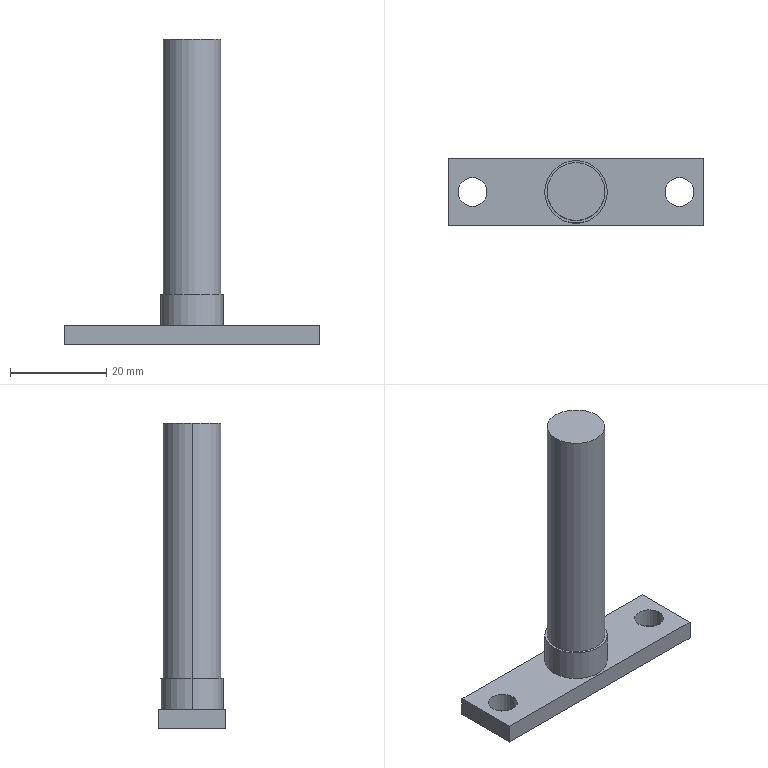Part | SolidWorks | features ICE 2, Extrusion 1 | 1 solid | 16 faces | box 53 x 14 x 63.5 mm | volume 9599 mm3 | cylinder 8 | plane 8 | commonest cylinder face diameters 6 x4 12 x2 13 x2
STEP:
#1=CARTESIAN_POINT('',(6.,0.,59.5));
#2=VERTEX_POINT('',#1);
#3=CARTESIAN_POINT('',(-6.,0.,59.5));
#4=VERTEX_POINT('',#3);
#5=CARTESIAN_POINT('',(0.,0.,59.5));
#6=DIRECTION('',(0.,0.,1.));
#7=DIRECTION('',(1.,0.,0.));
#8=AXIS2_PLACEMENT_3D('',#5,#6,#7);
#9=CIRCLE('',#8,6.);
#10=EDGE_CURVE('',#2,#4,#9,.T.);
#11=ORIENTED_EDGE('',*,*,#10,.F.);
#12=CARTESIAN_POINT('',(6.,0.,6.5));
#13=VERTEX_POINT('',#12);
#14=CARTESIAN_POINT('',(6.,0.,59.5));
#15=DIRECTION('',(0.,0.,-1.));
#16=VECTOR('',#15,1000.);
#17=LINE('',#14,#16);
#18=EDGE_CURVE('',#2,#13,#17,.T.);
#19=ORIENTED_EDGE('',*,*,#18,.T.);
#20=CARTESIAN_POINT('',(-6.,0.,6.5));
#21=VERTEX_POINT('',#20);
#22=CARTESIAN_POINT('',(0.,0.,6.5));
#23=DIRECTION('',(0.,0.,1.));
#24=DIRECTION('',(1.,0.,0.));
#25=AXIS2_PLACEMENT_3D('',#22,#23,#24);
#26=CIRCLE('',#25,6.);
#27=EDGE_CURVE('',#13,#21,#26,.T.);
#28=ORIENTED_EDGE('',*,*,#27,.T.);
#29=CARTESIAN_POINT('',(-6.,0.,59.5));
#30=DIRECTION('',(0.,0.,-1.));
#31=VECTOR('',#30,1000.);
#32=LINE('',#29,#31);
#33=EDGE_CURVE('',#4,#21,#32,.T.);
#34=ORIENTED_EDGE('',*,*,#33,.F.);
#35=EDGE_LOOP('',(#11,#19,#28,#34));
#36=FACE_OUTER_BOUND('',#35,.T.);
#37=CARTESIAN_POINT('',(0.,0.,59.5));
#38=DIRECTION('',(0.,0.,-1.));
#39=DIRECTION('',(-1.,0.,0.));
#40=AXIS2_PLACEMENT_3D('',#37,#38,#39);
#41=CYLINDRICAL_SURFACE('',#40,6.);
#42=ADVANCED_FACE('',(#36),#41,.T.);
#43=CARTESIAN_POINT('',(6.5,0.,6.5));
#44=VERTEX_POINT('',#43);
#45=CARTESIAN_POINT('',(-6.5,0.,6.5));
#46=VERTEX_POINT('',#45);
#47=CARTESIAN_POINT('',(0.,0.,6.5));
#48=DIRECTION('',(0.,0.,1.));
#49=DIRECTION('',(1.,0.,0.));
#50=AXIS2_PLACEMENT_3D('',#47,#48,#49);
#51=CIRCLE('',#50,6.5);
#52=EDGE_CURVE('',#44,#46,#51,.T.);
#53=ORIENTED_EDGE('',*,*,#52,.F.);
#54=CARTESIAN_POINT('',(6.5,0.,0.));
#55=VERTEX_POINT('',#54);
#56=CARTESIAN_POINT('',(6.5,0.,6.5));
#57=DIRECTION('',(0.,0.,-1.));
#58=VECTOR('',#57,1000.);
#59=LINE('',#56,#58);
#60=EDGE_CURVE('',#44,#55,#59,.T.);
#61=ORIENTED_EDGE('',*,*,#60,.T.);
#62=CARTESIAN_POINT('',(-6.5,0.,0.));
#63=VERTEX_POINT('',#62);
#64=CARTESIAN_POINT('',(0.,0.,0.));
#65=DIRECTION('',(0.,0.,1.));
#66=DIRECTION('',(1.,0.,0.));
#67=AXIS2_PLACEMENT_3D('',#64,#65,#66);
#68=CIRCLE('',#67,6.5);
#69=EDGE_CURVE('',#55,#63,#68,.T.);
#70=ORIENTED_EDGE('',*,*,#69,.T.);
#71=CARTESIAN_POINT('',(-6.5,0.,6.5));
#72=DIRECTION('',(0.,0.,-1.));
#73=VECTOR('',#72,1000.);
#74=LINE('',#71,#73);
#75=EDGE_CURVE('',#46,#63,#74,.T.);
#76=ORIENTED_EDGE('',*,*,#75,.F.);
#77=EDGE_LOOP('',(#53,#61,#70,#76));
#78=FACE_OUTER_BOUND('',#77,.T.);
#79=CARTESIAN_POINT('',(0.,0.,6.5));
#80=DIRECTION('',(0.,0.,-1.));
#81=DIRECTION('',(-1.,0.,0.));
#82=AXIS2_PLACEMENT_3D('',#79,#80,#81);
#83=CYLINDRICAL_SURFACE('',#82,6.5);
#84=ADVANCED_FACE('',(#78),#83,.T.);
#85=CARTESIAN_POINT('',(-18.5,0.,-4.));
#86=VERTEX_POINT('',#85);
#87=CARTESIAN_POINT('',(-24.5,0.,-4.));
#88=VERTEX_POINT('',#87);
#89=CARTESIAN_POINT('',(-21.5,0.,-4.));
#90=DIRECTION('',(0.,0.,-1.));
#91=DIRECTION('',(-1.,0.,0.));
#92=AXIS2_PLACEMENT_3D('',#89,#90,#91);
#93=CIRCLE('',#92,3.);
#94=EDGE_CURVE('',#86,#88,#93,.T.);
#95=ORIENTED_EDGE('',*,*,#94,.T.);
#96=CARTESIAN_POINT('',(-24.5,0.,0.));
#97=VERTEX_POINT('',#96);
#98=CARTESIAN_POINT('',(-24.5,0.,-4.));
#99=DIRECTION('',(0.,0.,1.));
#100=VECTOR('',#99,1000.);
#101=LINE('',#98,#100);
#102=EDGE_CURVE('',#88,#97,#101,.T.);
#103=ORIENTED_EDGE('',*,*,#102,.T.);
#104=CARTESIAN_POINT('',(-18.5,0.,0.));
#105=VERTEX_POINT('',#104);
#106=CARTESIAN_POINT('',(-21.5,0.,0.));
#107=DIRECTION('',(0.,0.,-1.));
#108=DIRECTION('',(-1.,0.,0.));
#109=AXIS2_PLACEMENT_3D('',#106,#107,#108);
#110=CIRCLE('',#109,3.);
#111=EDGE_CURVE('',#105,#97,#110,.T.);
#112=ORIENTED_EDGE('',*,*,#111,.F.);
#113=CARTESIAN_POINT('',(-18.5,0.,-4.));
#114=DIRECTION('',(0.,0.,1.));
#115=VECTOR('',#114,1000.);
#116=LINE('',#113,#115);
#117=EDGE_CURVE('',#86,#105,#116,.T.);
#118=ORIENTED_EDGE('',*,*,#117,.F.);
#119=EDGE_LOOP('',(#95,#103,#112,#118));
#120=FACE_OUTER_BOUND('',#119,.T.);
#121=CARTESIAN_POINT('',(-21.5,0.,-4.));
#122=DIRECTION('',(0.,0.,1.));
#123=DIRECTION('',(1.,0.,0.));
#124=AXIS2_PLACEMENT_3D('',#121,#122,#123);
#125=CYLINDRICAL_SURFACE('',#124,3.);
#126=ADVANCED_FACE('',(#120),#125,.F.);
#127=CARTESIAN_POINT('',(24.5,0.,-4.));
#128=VERTEX_POINT('',#127);
#129=CARTESIAN_POINT('',(18.5,0.,-4.));
#130=VERTEX_POINT('',#129);
#131=CARTESIAN_POINT('',(21.5,0.,-4.));
#132=DIRECTION('',(0.,0.,-1.));
#133=DIRECTION('',(-1.,0.,0.));
#134=AXIS2_PLACEMENT_3D('',#131,#132,#133);
#135=CIRCLE('',#134,3.);
#136=EDGE_CURVE('',#128,#130,#135,.T.);
#137=ORIENTED_EDGE('',*,*,#136,.T.);
#138=CARTESIAN_POINT('',(18.5,0.,0.));
#139=VERTEX_POINT('',#138);
#140=CARTESIAN_POINT('',(18.5,0.,-4.));
#141=DIRECTION('',(0.,0.,1.));
#142=VECTOR('',#141,1000.);
#143=LINE('',#140,#142);
#144=EDGE_CURVE('',#130,#139,#143,.T.);
#145=ORIENTED_EDGE('',*,*,#144,.T.);
#146=CARTESIAN_POINT('',(24.5,0.,0.));
#147=VERTEX_POINT('',#146);
#148=CARTESIAN_POINT('',(21.5,0.,0.));
#149=DIRECTION('',(0.,0.,-1.));
#150=DIRECTION('',(-1.,0.,0.));
#151=AXIS2_PLACEMENT_3D('',#148,#149,#150);
#152=CIRCLE('',#151,3.);
#153=EDGE_CURVE('',#147,#139,#152,.T.);
#154=ORIENTED_EDGE('',*,*,#153,.F.);
#155=CARTESIAN_POINT('',(24.5,0.,-4.));
#156=DIRECTION('',(0.,0.,1.));
#157=VECTOR('',#156,1000.);
#158=LINE('',#155,#157);
#159=EDGE_CURVE('',#128,#147,#158,.T.);
#160=ORIENTED_EDGE('',*,*,#159,.F.);
#161=EDGE_LOOP('',(#137,#145,#154,#160));
#162=FACE_OUTER_BOUND('',#161,.T.);
#163=CARTESIAN_POINT('',(21.5,0.,-4.));
#164=DIRECTION('',(0.,0.,1.));
#165=DIRECTION('',(1.,0.,0.));
#166=AXIS2_PLACEMENT_3D('',#163,#164,#165);
#167=CYLINDRICAL_SURFACE('',#166,3.);
#168=ADVANCED_FACE('',(#162),#167,.F.);
#169=CARTESIAN_POINT('',(-26.5,-7.,-4.));
#170=VERTEX_POINT('',#169);
#171=CARTESIAN_POINT('',(-26.5,7.,-4.));
#172=VERTEX_POINT('',#171);
#173=CARTESIAN_POINT('',(-26.5,-7.,-4.));
#174=DIRECTION('',(0.,1.,0.));
#175=VECTOR('',#174,1000.);
#176=LINE('',#173,#175);
#177=EDGE_CURVE('',#170,#172,#176,.T.);
#178=ORIENTED_EDGE('',*,*,#177,.T.);
#179=CARTESIAN_POINT('',(26.5,7.,-4.));
#180=VERTEX_POINT('',#179);
#181=CARTESIAN_POINT('',(26.5,7.,-4.));
#182=DIRECTION('',(1.,0.,0.));
#183=VECTOR('',#182,1000.);
#184=LINE('',#181,#183);
#185=EDGE_CURVE('',#172,#180,#184,.T.);
#186=ORIENTED_EDGE('',*,*,#185,.T.);
#187=CARTESIAN_POINT('',(26.5,-7.,-4.));
#188=VERTEX_POINT('',#187);
#189=CARTESIAN_POINT('',(26.5,-7.,-4.));
#190=DIRECTION('',(0.,-1.,0.));
#191=VECTOR('',#190,1000.);
#192=LINE('',#189,#191);
#193=EDGE_CURVE('',#180,#188,#192,.T.);
#194=ORIENTED_EDGE('',*,*,#193,.T.);
#195=CARTESIAN_POINT('',(26.5,-7.,-4.));
#196=DIRECTION('',(-1.,0.,0.));
#197=VECTOR('',#196,1000.);
#198=LINE('',#195,#197);
#199=EDGE_CURVE('',#188,#170,#198,.T.);
#200=ORIENTED_EDGE('',*,*,#199,.T.);
#201=EDGE_LOOP('',(#178,#186,#194,#200));
#202=FACE_OUTER_BOUND('',#201,.T.);
#203=ORIENTED_EDGE('',*,*,#136,.F.);
#204=CARTESIAN_POINT('',(21.5,0.,-4.));
#205=DIRECTION('',(0.,0.,-1.));
#206=DIRECTION('',(-1.,0.,0.));
#207=AXIS2_PLACEMENT_3D('',#204,#205,#206);
#208=CIRCLE('',#207,3.);
#209=EDGE_CURVE('',#130,#128,#208,.T.);
#210=ORIENTED_EDGE('',*,*,#209,.F.);
#211=EDGE_LOOP('',(#203,#210));
#212=FACE_BOUND('',#211,.T.);
#213=ORIENTED_EDGE('',*,*,#94,.F.);
#214=CARTESIAN_POINT('',(-21.5,0.,-4.));
#215=DIRECTION('',(0.,0.,-1.));
#216=DIRECTION('',(-1.,0.,0.));
#217=AXIS2_PLACEMENT_3D('',#214,#215,#216);
#218=CIRCLE('',#217,3.);
#219=EDGE_CURVE('',#88,#86,#218,.T.);
#220=ORIENTED_EDGE('',*,*,#219,.F.);
#221=EDGE_LOOP('',(#213,#220));
#222=FACE_BOUND('',#221,.T.);
#223=CARTESIAN_POINT('',(0.,0.,-4.));
#224=DIRECTION('',(0.,0.,1.));
#225=DIRECTION('',(1.,0.,0.));
#226=AXIS2_PLACEMENT_3D('',#223,#224,#225);
#227=PLANE('',#226);
#228=ADVANCED_FACE('',(#202,#212,#222),#227,.F.);
#229=CARTESIAN_POINT('',(0.,0.,0.));
#230=DIRECTION('',(0.,0.,1.));
#231=DIRECTION('',(1.,0.,0.));
#232=AXIS2_PLACEMENT_3D('',#229,#230,#231);
#233=CIRCLE('',#232,6.5);
#234=EDGE_CURVE('',#63,#55,#233,.T.);
#235=ORIENTED_EDGE('',*,*,#234,.F.);
#236=ORIENTED_EDGE('',*,*,#69,.F.);
#237=EDGE_LOOP('',(#235,#236));
#238=FACE_BOUND('',#237,.T.);
#239=ORIENTED_EDGE('',*,*,#153,.T.);
#240=CARTESIAN_POINT('',(21.5,0.,0.));
#241=DIRECTION('',(0.,0.,-1.));
#242=DIRECTION('',(-1.,0.,0.));
#243=AXIS2_PLACEMENT_3D('',#240,#241,#242);
#244=CIRCLE('',#243,3.);
#245=EDGE_CURVE('',#139,#147,#244,.T.);
#246=ORIENTED_EDGE('',*,*,#245,.T.);
#247=EDGE_LOOP('',(#239,#246));
#248=FACE_BOUND('',#247,.T.);
#249=CARTESIAN_POINT('',(-26.5,-7.,0.));
#250=VERTEX_POINT('',#249);
#251=CARTESIAN_POINT('',(-26.5,7.,0.));
#252=VERTEX_POINT('',#251);
#253=CARTESIAN_POINT('',(-26.5,-7.,0.));
#254=DIRECTION('',(0.,1.,0.));
#255=VECTOR('',#254,1000.);
#256=LINE('',#253,#255);
#257=EDGE_CURVE('',#250,#252,#256,.T.);
#258=ORIENTED_EDGE('',*,*,#257,.F.);
#259=CARTESIAN_POINT('',(26.5,-7.,0.));
#260=VERTEX_POINT('',#259);
#261=CARTESIAN_POINT('',(26.5,-7.,0.));
#262=DIRECTION('',(-1.,0.,0.));
#263=VECTOR('',#262,1000.);
#264=LINE('',#261,#263);
#265=EDGE_CURVE('',#260,#250,#264,.T.);
#266=ORIENTED_EDGE('',*,*,#265,.F.);
#267=CARTESIAN_POINT('',(26.5,7.,0.));
#268=VERTEX_POINT('',#267);
#269=CARTESIAN_POINT('',(26.5,-7.,0.));
#270=DIRECTION('',(0.,-1.,0.));
#271=VECTOR('',#270,1000.);
#272=LINE('',#269,#271);
#273=EDGE_CURVE('',#268,#260,#272,.T.);
#274=ORIENTED_EDGE('',*,*,#273,.F.);
#275=CARTESIAN_POINT('',(26.5,7.,0.));
#276=DIRECTION('',(1.,0.,0.));
#277=VECTOR('',#276,1000.);
#278=LINE('',#275,#277);
#279=EDGE_CURVE('',#252,#268,#278,.T.);
#280=ORIENTED_EDGE('',*,*,#279,.F.);
#281=EDGE_LOOP('',(#258,#266,#274,#280));
#282=FACE_OUTER_BOUND('',#281,.T.);
#283=ORIENTED_EDGE('',*,*,#111,.T.);
#284=CARTESIAN_POINT('',(-21.5,0.,0.));
#285=DIRECTION('',(0.,0.,-1.));
#286=DIRECTION('',(-1.,0.,0.));
#287=AXIS2_PLACEMENT_3D('',#284,#285,#286);
#288=CIRCLE('',#287,3.);
#289=EDGE_CURVE('',#97,#105,#288,.T.);
#290=ORIENTED_EDGE('',*,*,#289,.T.);
#291=EDGE_LOOP('',(#283,#290));
#292=FACE_BOUND('',#291,.T.);
#293=CARTESIAN_POINT('',(0.,0.,0.));
#294=DIRECTION('',(0.,0.,1.));
#295=DIRECTION('',(1.,0.,0.));
#296=AXIS2_PLACEMENT_3D('',#293,#294,#295);
#297=PLANE('',#296);
#298=ADVANCED_FACE('',(#238,#248,#282,#292),#297,.T.);
#299=ORIENTED_EDGE('',*,*,#257,.T.);
#300=CARTESIAN_POINT('',(-26.5,7.,-4.));
#301=DIRECTION('',(0.,0.,1.));
#302=VECTOR('',#301,1000.);
#303=LINE('',#300,#302);
#304=EDGE_CURVE('',#172,#252,#303,.T.);
#305=ORIENTED_EDGE('',*,*,#304,.F.);
#306=ORIENTED_EDGE('',*,*,#177,.F.);
#307=CARTESIAN_POINT('',(-26.5,-7.,-4.));
#308=DIRECTION('',(0.,0.,1.));
#309=VECTOR('',#308,1000.);
#310=LINE('',#307,#309);
#311=EDGE_CURVE('',#170,#250,#310,.T.);
#312=ORIENTED_EDGE('',*,*,#311,.T.);
#313=EDGE_LOOP('',(#299,#305,#306,#312));
#314=FACE_OUTER_BOUND('',#313,.T.);
#315=CARTESIAN_POINT('',(-26.5,-7.,-4.));
#316=DIRECTION('',(1.,0.,0.));
#317=DIRECTION('',(0.,0.,-1.));
#318=AXIS2_PLACEMENT_3D('',#315,#316,#317);
#319=PLANE('',#318);
#320=ADVANCED_FACE('',(#314),#319,.F.);
#321=ORIENTED_EDGE('',*,*,#279,.T.);
#322=CARTESIAN_POINT('',(26.5,7.,-4.));
#323=DIRECTION('',(0.,0.,1.));
#324=VECTOR('',#323,1000.);
#325=LINE('',#322,#324);
#326=EDGE_CURVE('',#180,#268,#325,.T.);
#327=ORIENTED_EDGE('',*,*,#326,.F.);
#328=ORIENTED_EDGE('',*,*,#185,.F.);
#329=ORIENTED_EDGE('',*,*,#304,.T.);
#330=EDGE_LOOP('',(#321,#327,#328,#329));
#331=FACE_OUTER_BOUND('',#330,.T.);
#332=CARTESIAN_POINT('',(26.5,7.,-4.));
#333=DIRECTION('',(0.,-1.,0.));
#334=DIRECTION('',(0.,0.,-1.));
#335=AXIS2_PLACEMENT_3D('',#332,#333,#334);
#336=PLANE('',#335);
#337=ADVANCED_FACE('',(#331),#336,.F.);
#338=ORIENTED_EDGE('',*,*,#273,.T.);
#339=CARTESIAN_POINT('',(26.5,-7.,-4.));
#340=DIRECTION('',(0.,0.,1.));
#341=VECTOR('',#340,1000.);
#342=LINE('',#339,#341);
#343=EDGE_CURVE('',#188,#260,#342,.T.);
#344=ORIENTED_EDGE('',*,*,#343,.F.);
#345=ORIENTED_EDGE('',*,*,#193,.F.);
#346=ORIENTED_EDGE('',*,*,#326,.T.);
#347=EDGE_LOOP('',(#338,#344,#345,#346));
#348=FACE_OUTER_BOUND('',#347,.T.);
#349=CARTESIAN_POINT('',(26.5,-7.,-4.));
#350=DIRECTION('',(-1.,0.,0.));
#351=DIRECTION('',(0.,0.,1.));
#352=AXIS2_PLACEMENT_3D('',#349,#350,#351);
#353=PLANE('',#352);
#354=ADVANCED_FACE('',(#348),#353,.F.);
#355=ORIENTED_EDGE('',*,*,#265,.T.);
#356=ORIENTED_EDGE('',*,*,#311,.F.);
#357=ORIENTED_EDGE('',*,*,#199,.F.);
#358=ORIENTED_EDGE('',*,*,#343,.T.);
#359=EDGE_LOOP('',(#355,#356,#357,#358));
#360=FACE_OUTER_BOUND('',#359,.T.);
#361=CARTESIAN_POINT('',(26.5,-7.,-4.));
#362=DIRECTION('',(0.,1.,0.));
#363=DIRECTION('',(0.,0.,1.));
#364=AXIS2_PLACEMENT_3D('',#361,#362,#363);
#365=PLANE('',#364);
#366=ADVANCED_FACE('',(#360),#365,.F.);
#367=ORIENTED_EDGE('',*,*,#144,.F.);
#368=ORIENTED_EDGE('',*,*,#209,.T.);
#369=ORIENTED_EDGE('',*,*,#159,.T.);
#370=ORIENTED_EDGE('',*,*,#245,.F.);
#371=EDGE_LOOP('',(#367,#368,#369,#370));
#372=FACE_OUTER_BOUND('',#371,.T.);
#373=CARTESIAN_POINT('',(21.5,0.,-4.));
#374=DIRECTION('',(0.,0.,1.));
#375=DIRECTION('',(1.,0.,0.));
#376=AXIS2_PLACEMENT_3D('',#373,#374,#375);
#377=CYLINDRICAL_SURFACE('',#376,3.);
#378=ADVANCED_FACE('',(#372),#377,.F.);
#379=ORIENTED_EDGE('',*,*,#102,.F.);
#380=ORIENTED_EDGE('',*,*,#219,.T.);
#381=ORIENTED_EDGE('',*,*,#117,.T.);
#382=ORIENTED_EDGE('',*,*,#289,.F.);
#383=EDGE_LOOP('',(#379,#380,#381,#382));
#384=FACE_OUTER_BOUND('',#383,.T.);
#385=CARTESIAN_POINT('',(-21.5,0.,-4.));
#386=DIRECTION('',(0.,0.,1.));
#387=DIRECTION('',(1.,0.,0.));
#388=AXIS2_PLACEMENT_3D('',#385,#386,#387);
#389=CYLINDRICAL_SURFACE('',#388,3.);
#390=ADVANCED_FACE('',(#384),#389,.F.);
#391=ORIENTED_EDGE('',*,*,#60,.F.);
#392=CARTESIAN_POINT('',(0.,0.,6.5));
#393=DIRECTION('',(0.,0.,1.));
#394=DIRECTION('',(1.,0.,0.));
#395=AXIS2_PLACEMENT_3D('',#392,#393,#394);
#396=CIRCLE('',#395,6.5);
#397=EDGE_CURVE('',#46,#44,#396,.T.);
#398=ORIENTED_EDGE('',*,*,#397,.F.);
#399=ORIENTED_EDGE('',*,*,#75,.T.);
#400=ORIENTED_EDGE('',*,*,#234,.T.);
#401=EDGE_LOOP('',(#391,#398,#399,#400));
#402=FACE_OUTER_BOUND('',#401,.T.);
#403=CARTESIAN_POINT('',(0.,0.,6.5));
#404=DIRECTION('',(0.,0.,-1.));
#405=DIRECTION('',(-1.,0.,0.));
#406=AXIS2_PLACEMENT_3D('',#403,#404,#405);
#407=CYLINDRICAL_SURFACE('',#406,6.5);
#408=ADVANCED_FACE('',(#402),#407,.T.);
#409=CARTESIAN_POINT('',(0.,0.,6.5));
#410=DIRECTION('',(0.,0.,1.));
#411=DIRECTION('',(1.,0.,0.));
#412=AXIS2_PLACEMENT_3D('',#409,#410,#411);
#413=CIRCLE('',#412,6.);
#414=EDGE_CURVE('',#21,#13,#413,.T.);
#415=ORIENTED_EDGE('',*,*,#414,.F.);
#416=ORIENTED_EDGE('',*,*,#27,.F.);
#417=EDGE_LOOP('',(#415,#416));
#418=FACE_BOUND('',#417,.T.);
#419=ORIENTED_EDGE('',*,*,#397,.T.);
#420=ORIENTED_EDGE('',*,*,#52,.T.);
#421=EDGE_LOOP('',(#419,#420));
#422=FACE_OUTER_BOUND('',#421,.T.);
#423=CARTESIAN_POINT('',(0.,0.,6.5));
#424=DIRECTION('',(0.,0.,1.));
#425=DIRECTION('',(1.,0.,0.));
#426=AXIS2_PLACEMENT_3D('',#423,#424,#425);
#427=PLANE('',#426);
#428=ADVANCED_FACE('',(#418,#422),#427,.T.);
#429=CARTESIAN_POINT('',(0.,0.,59.5));
#430=DIRECTION('',(0.,0.,1.));
#431=DIRECTION('',(1.,0.,0.));
#432=AXIS2_PLACEMENT_3D('',#429,#430,#431);
#433=CIRCLE('',#432,6.);
#434=EDGE_CURVE('',#4,#2,#433,.T.);
#435=ORIENTED_EDGE('',*,*,#434,.T.);
#436=ORIENTED_EDGE('',*,*,#10,.T.);
#437=EDGE_LOOP('',(#435,#436));
#438=FACE_OUTER_BOUND('',#437,.T.);
#439=CARTESIAN_POINT('',(0.,0.,59.5));
#440=DIRECTION('',(0.,0.,1.));
#441=DIRECTION('',(1.,0.,0.));
#442=AXIS2_PLACEMENT_3D('',#439,#440,#441);
#443=PLANE('',#442);
#444=ADVANCED_FACE('',(#438),#443,.T.);
#445=ORIENTED_EDGE('',*,*,#18,.F.);
#446=ORIENTED_EDGE('',*,*,#434,.F.);
#447=ORIENTED_EDGE('',*,*,#33,.T.);
#448=ORIENTED_EDGE('',*,*,#414,.T.);
#449=EDGE_LOOP('',(#445,#446,#447,#448));
#450=FACE_OUTER_BOUND('',#449,.T.);
#451=CARTESIAN_POINT('',(0.,0.,59.5));
#452=DIRECTION('',(0.,0.,-1.));
#453=DIRECTION('',(-1.,0.,0.));
#454=AXIS2_PLACEMENT_3D('',#451,#452,#453);
#455=CYLINDRICAL_SURFACE('',#454,6.);
#456=ADVANCED_FACE('',(#450),#455,.T.);
#457=CLOSED_SHELL('',(#42,#84,#126,#168,#228,#298,#320,#337,#354,#366,#378,#390,#408,#428,#444,#456));
#458=MANIFOLD_SOLID_BREP('',#457);
#459=CARTESIAN_POINT('',(0.,0.,0.));
#460=DIRECTION('',(0.,0.,1.));
#461=DIRECTION('',(1.,0.,0.));
#462=AXIS2_PLACEMENT_3D('',#459,#460,#461);
#463=(LENGTH_UNIT()NAMED_UNIT(*)SI_UNIT(.MILLI.,.METRE.));
#464=UNCERTAINTY_MEASURE_WITH_UNIT(LENGTH_MEASURE(0.00001),#463,'','');
#465=(NAMED_UNIT(*)PLANE_ANGLE_UNIT()SI_UNIT($,.RADIAN.));
#466=(NAMED_UNIT(*)SI_UNIT($,.STERADIAN.)SOLID_ANGLE_UNIT());
#467=(GEOMETRIC_REPRESENTATION_CONTEXT(3)GLOBAL_UNCERTAINTY_ASSIGNED_CONTEXT((#464))GLOBAL_UNIT_ASSIGNED_CONTEXT((#463,#465,#466))REPRESENTATION_CONTEXT('',''));
#468=ADVANCED_BREP_SHAPE_REPRESENTATION('',(#458,#462),#467);